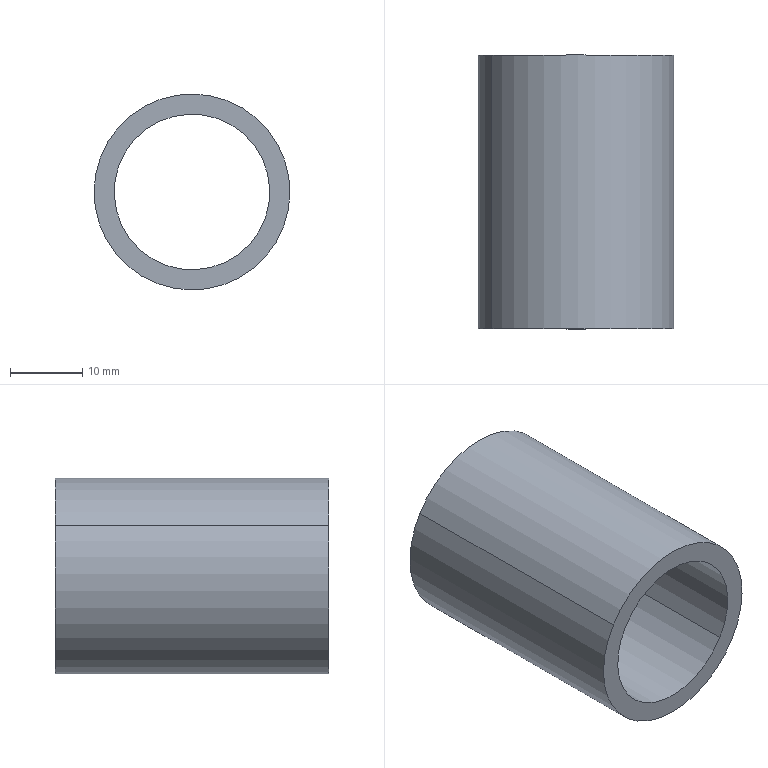Part | STEP file | [02]-12 | 1 solid | 6 faces | box 27.2 x 38 x 27.2 mm | volume 8156 mm3 | cylinder 4 | plane 2 | commonest cylinder face diameters 21.6 x2 27.2 x2
STEP:
#1=CARTESIAN_POINT('',(0.,0.,0.));
#2=DIRECTION('',(0.,0.,1.));
#3=DIRECTION('',(1.,0.,0.));
#4=AXIS2_PLACEMENT_3D('',#1,#2,#3);
#5=CARTESIAN_POINT('',(9.263,20.,-5.553));
#6=VERTEX_POINT('',#5);
#7=CARTESIAN_POINT('',(9.263,-18.,-5.553));
#8=VERTEX_POINT('',#7);
#9=CARTESIAN_POINT('',(9.263,20.,-5.553));
#10=DIRECTION('',(0.,-1.,0.));
#11=VECTOR('',#10,1.);
#12=LINE('',#9,#11);
#13=CARTESIAN_POINT('',(0.,20.,0.));
#14=DIRECTION('',(0.,-1.,0.));
#15=DIRECTION('',(0.8577,0.,-0.5142));
#16=AXIS2_PLACEMENT_3D('',#13,#14,#15);
#17=CYLINDRICAL_SURFACE('',#16,10.8);
#18=CARTESIAN_POINT('',(6.283,0.));
#19=DIRECTION('',(0.,1.));
#20=VECTOR('',#19,1.);
#21=LINE('',#18,#20);
#22=(GEOMETRIC_REPRESENTATION_CONTEXT(2)PARAMETRIC_REPRESENTATION_CONTEXT()REPRESENTATION_CONTEXT('',''));
#23=DEFINITIONAL_REPRESENTATION('',(#21),#22);
#24=PCURVE('',#17,#23);
#25=CARTESIAN_POINT('',(0.,20.,0.));
#26=DIRECTION('',(0.,-1.,0.));
#27=DIRECTION('',(0.8577,0.,-0.5142));
#28=AXIS2_PLACEMENT_3D('',#25,#26,#27);
#29=CYLINDRICAL_SURFACE('',#28,10.8);
#30=CARTESIAN_POINT('',(0.,0.));
#31=DIRECTION('',(0.,1.));
#32=VECTOR('',#31,1.);
#33=LINE('',#30,#32);
#34=(GEOMETRIC_REPRESENTATION_CONTEXT(2)PARAMETRIC_REPRESENTATION_CONTEXT()REPRESENTATION_CONTEXT('',''));
#35=DEFINITIONAL_REPRESENTATION('',(#33),#34);
#36=PCURVE('',#29,#35);
#37=SURFACE_CURVE('',#12,(#24,#36),.PCURVE_S1.);
#38=EDGE_CURVE('',#6,#8,#37,.T.);
#39=ORIENTED_EDGE('',*,*,#38,.T.);
#40=CARTESIAN_POINT('',(-9.263,-18.,5.553));
#41=VERTEX_POINT('',#40);
#42=CARTESIAN_POINT('',(0.,-18.,0.));
#43=DIRECTION('',(0.,1.,0.));
#44=DIRECTION('',(-0.8577,0.,0.5142));
#45=AXIS2_PLACEMENT_3D('',#42,#43,#44);
#46=CIRCLE('',#45,10.8);
#47=CARTESIAN_POINT('',(9.425,38.));
#48=DIRECTION('',(-1.,0.));
#49=VECTOR('',#48,1.);
#50=LINE('',#47,#49);
#51=(GEOMETRIC_REPRESENTATION_CONTEXT(2)PARAMETRIC_REPRESENTATION_CONTEXT()REPRESENTATION_CONTEXT('',''));
#52=DEFINITIONAL_REPRESENTATION('',(#50),#51);
#53=PCURVE('',#17,#52);
#54=CARTESIAN_POINT('',(0.,-18.,0.));
#55=DIRECTION('',(0.,-1.,0.));
#56=DIRECTION('',(0.8577,0.,-0.5142));
#57=AXIS2_PLACEMENT_3D('',#54,#55,#56);
#58=PLANE('',#57);
#59=CARTESIAN_POINT('',(-10.8,0.));
#60=CARTESIAN_POINT('',(-10.8,18.706));
#61=CARTESIAN_POINT('',(5.4,9.353));
#62=CARTESIAN_POINT('',(21.6,0.));
#63=CARTESIAN_POINT('',(5.4,-9.353));
#64=CARTESIAN_POINT('',(-10.8,-18.706));
#65=CARTESIAN_POINT('',(-10.8,0.));
#66=(BOUNDED_CURVE()B_SPLINE_CURVE(2,(#59,#60,#61,#62,#63,#64,#65),.UNSPECIFIED.,.T.,.F.)B_SPLINE_CURVE_WITH_KNOTS((1,2,2,2,2,1),(-2.094,0.,2.094,4.189,6.283,8.378),.UNSPECIFIED.)CURVE()GEOMETRIC_REPRESENTATION_ITEM()RATIONAL_B_SPLINE_CURVE((1.,0.5,1.,0.5,1.,0.5,1.))REPRESENTATION_ITEM(''));
#67=(GEOMETRIC_REPRESENTATION_CONTEXT(2)PARAMETRIC_REPRESENTATION_CONTEXT()REPRESENTATION_CONTEXT('',''));
#68=DEFINITIONAL_REPRESENTATION('',(#66),#67);
#69=PCURVE('',#58,#68);
#70=SURFACE_CURVE('',#46,(#53,#69),.PCURVE_S1.);
#71=EDGE_CURVE('',#8,#41,#70,.T.);
#72=ORIENTED_EDGE('',*,*,#71,.T.);
#73=CARTESIAN_POINT('',(-9.263,20.,5.553));
#74=VERTEX_POINT('',#73);
#75=CARTESIAN_POINT('',(-9.263,20.,5.553));
#76=DIRECTION('',(0.,-1.,0.));
#77=VECTOR('',#76,1.);
#78=LINE('',#75,#77);
#79=CARTESIAN_POINT('',(3.142,0.));
#80=DIRECTION('',(0.,1.));
#81=VECTOR('',#80,1.);
#82=LINE('',#79,#81);
#83=(GEOMETRIC_REPRESENTATION_CONTEXT(2)PARAMETRIC_REPRESENTATION_CONTEXT()REPRESENTATION_CONTEXT('',''));
#84=DEFINITIONAL_REPRESENTATION('',(#82),#83);
#85=PCURVE('',#17,#84);
#86=CARTESIAN_POINT('',(3.142,0.));
#87=DIRECTION('',(0.,1.));
#88=VECTOR('',#87,1.);
#89=LINE('',#86,#88);
#90=(GEOMETRIC_REPRESENTATION_CONTEXT(2)PARAMETRIC_REPRESENTATION_CONTEXT()REPRESENTATION_CONTEXT('',''));
#91=DEFINITIONAL_REPRESENTATION('',(#89),#90);
#92=PCURVE('',#29,#91);
#93=SURFACE_CURVE('',#78,(#85,#92),.PCURVE_S1.);
#94=EDGE_CURVE('',#74,#41,#93,.T.);
#95=ORIENTED_EDGE('',*,*,#94,.F.);
#96=CARTESIAN_POINT('',(0.,20.,0.));
#97=DIRECTION('',(0.,-1.,0.));
#98=DIRECTION('',(0.8577,0.,-0.5142));
#99=AXIS2_PLACEMENT_3D('',#96,#97,#98);
#100=CIRCLE('',#99,10.8);
#101=CARTESIAN_POINT('',(0.,0.));
#102=DIRECTION('',(1.,0.));
#103=VECTOR('',#102,1.);
#104=LINE('',#101,#103);
#105=(GEOMETRIC_REPRESENTATION_CONTEXT(2)PARAMETRIC_REPRESENTATION_CONTEXT()REPRESENTATION_CONTEXT('',''));
#106=DEFINITIONAL_REPRESENTATION('',(#104),#105);
#107=PCURVE('',#17,#106);
#108=CARTESIAN_POINT('',(0.,20.,0.));
#109=DIRECTION('',(0.,1.,0.));
#110=DIRECTION('',(-0.8577,0.,0.5142));
#111=AXIS2_PLACEMENT_3D('',#108,#109,#110);
#112=PLANE('',#111);
#113=CARTESIAN_POINT('',(-10.8,0.));
#114=CARTESIAN_POINT('',(-10.8,18.706));
#115=CARTESIAN_POINT('',(5.4,9.353));
#116=CARTESIAN_POINT('',(21.6,0.));
#117=CARTESIAN_POINT('',(5.4,-9.353));
#118=CARTESIAN_POINT('',(-10.8,-18.706));
#119=CARTESIAN_POINT('',(-10.8,0.));
#120=(BOUNDED_CURVE()B_SPLINE_CURVE(2,(#113,#114,#115,#116,#117,#118,#119),.UNSPECIFIED.,.T.,.F.)B_SPLINE_CURVE_WITH_KNOTS((1,2,2,2,2,1),(-2.094,0.,2.094,4.189,6.283,8.378),.UNSPECIFIED.)CURVE()GEOMETRIC_REPRESENTATION_ITEM()RATIONAL_B_SPLINE_CURVE((1.,0.5,1.,0.5,1.,0.5,1.))REPRESENTATION_ITEM(''));
#121=(GEOMETRIC_REPRESENTATION_CONTEXT(2)PARAMETRIC_REPRESENTATION_CONTEXT()REPRESENTATION_CONTEXT('',''));
#122=DEFINITIONAL_REPRESENTATION('',(#120),#121);
#123=PCURVE('',#112,#122);
#124=SURFACE_CURVE('',#100,(#107,#123),.PCURVE_S1.);
#125=EDGE_CURVE('',#74,#6,#124,.T.);
#126=ORIENTED_EDGE('',*,*,#125,.T.);
#127=EDGE_LOOP('',(#39,#72,#95,#126));
#128=FACE_BOUND('',#127,.F.);
#129=ADVANCED_FACE('',(#128),#17,.F.);
#130=CARTESIAN_POINT('',(11.665,20.,-6.993));
#131=VERTEX_POINT('',#130);
#132=CARTESIAN_POINT('',(-11.665,20.,6.993));
#133=VERTEX_POINT('',#132);
#134=CARTESIAN_POINT('',(0.,20.,0.));
#135=DIRECTION('',(0.,-1.,0.));
#136=DIRECTION('',(0.8577,0.,-0.5142));
#137=AXIS2_PLACEMENT_3D('',#134,#135,#136);
#138=CIRCLE('',#137,13.6);
#139=CARTESIAN_POINT('',(0.,20.,0.));
#140=DIRECTION('',(0.,-1.,0.));
#141=DIRECTION('',(0.8577,0.,-0.5142));
#142=AXIS2_PLACEMENT_3D('',#139,#140,#141);
#143=CYLINDRICAL_SURFACE('',#142,13.6);
#144=CARTESIAN_POINT('',(0.,0.));
#145=DIRECTION('',(1.,0.));
#146=VECTOR('',#145,1.);
#147=LINE('',#144,#146);
#148=(GEOMETRIC_REPRESENTATION_CONTEXT(2)PARAMETRIC_REPRESENTATION_CONTEXT()REPRESENTATION_CONTEXT('',''));
#149=DEFINITIONAL_REPRESENTATION('',(#147),#148);
#150=PCURVE('',#143,#149);
#151=CARTESIAN_POINT('',(-13.6,0.));
#152=CARTESIAN_POINT('',(-13.6,23.556));
#153=CARTESIAN_POINT('',(6.8,11.778));
#154=CARTESIAN_POINT('',(27.2,0.));
#155=CARTESIAN_POINT('',(6.8,-11.778));
#156=CARTESIAN_POINT('',(-13.6,-23.556));
#157=CARTESIAN_POINT('',(-13.6,0.));
#158=(BOUNDED_CURVE()B_SPLINE_CURVE(2,(#151,#152,#153,#154,#155,#156,#157),.UNSPECIFIED.,.T.,.F.)B_SPLINE_CURVE_WITH_KNOTS((1,2,2,2,2,1),(-2.094,0.,2.094,4.189,6.283,8.378),.UNSPECIFIED.)CURVE()GEOMETRIC_REPRESENTATION_ITEM()RATIONAL_B_SPLINE_CURVE((1.,0.5,1.,0.5,1.,0.5,1.))REPRESENTATION_ITEM(''));
#159=(GEOMETRIC_REPRESENTATION_CONTEXT(2)PARAMETRIC_REPRESENTATION_CONTEXT()REPRESENTATION_CONTEXT('',''));
#160=DEFINITIONAL_REPRESENTATION('',(#158),#159);
#161=PCURVE('',#112,#160);
#162=SURFACE_CURVE('',#138,(#150,#161),.PCURVE_S1.);
#163=EDGE_CURVE('',#131,#133,#162,.T.);
#164=ORIENTED_EDGE('',*,*,#163,.T.);
#165=CARTESIAN_POINT('',(-11.665,-18.,6.993));
#166=VERTEX_POINT('',#165);
#167=CARTESIAN_POINT('',(-11.665,20.,6.993));
#168=DIRECTION('',(0.,-1.,0.));
#169=VECTOR('',#168,1.);
#170=LINE('',#167,#169);
#171=CARTESIAN_POINT('',(3.142,0.));
#172=DIRECTION('',(0.,1.));
#173=VECTOR('',#172,1.);
#174=LINE('',#171,#173);
#175=(GEOMETRIC_REPRESENTATION_CONTEXT(2)PARAMETRIC_REPRESENTATION_CONTEXT()REPRESENTATION_CONTEXT('',''));
#176=DEFINITIONAL_REPRESENTATION('',(#174),#175);
#177=PCURVE('',#143,#176);
#178=CARTESIAN_POINT('',(0.,20.,0.));
#179=DIRECTION('',(0.,-1.,0.));
#180=DIRECTION('',(0.8577,0.,-0.5142));
#181=AXIS2_PLACEMENT_3D('',#178,#179,#180);
#182=CYLINDRICAL_SURFACE('',#181,13.6);
#183=CARTESIAN_POINT('',(3.142,0.));
#184=DIRECTION('',(0.,1.));
#185=VECTOR('',#184,1.);
#186=LINE('',#183,#185);
#187=(GEOMETRIC_REPRESENTATION_CONTEXT(2)PARAMETRIC_REPRESENTATION_CONTEXT()REPRESENTATION_CONTEXT('',''));
#188=DEFINITIONAL_REPRESENTATION('',(#186),#187);
#189=PCURVE('',#182,#188);
#190=SURFACE_CURVE('',#170,(#177,#189),.PCURVE_S1.);
#191=EDGE_CURVE('',#133,#166,#190,.T.);
#192=ORIENTED_EDGE('',*,*,#191,.T.);
#193=CARTESIAN_POINT('',(11.665,-18.,-6.993));
#194=VERTEX_POINT('',#193);
#195=CARTESIAN_POINT('',(0.,-18.,0.));
#196=DIRECTION('',(0.,1.,0.));
#197=DIRECTION('',(-0.8577,0.,0.5142));
#198=AXIS2_PLACEMENT_3D('',#195,#196,#197);
#199=CIRCLE('',#198,13.6);
#200=CARTESIAN_POINT('',(3.142,38.));
#201=DIRECTION('',(-1.,0.));
#202=VECTOR('',#201,1.);
#203=LINE('',#200,#202);
#204=(GEOMETRIC_REPRESENTATION_CONTEXT(2)PARAMETRIC_REPRESENTATION_CONTEXT()REPRESENTATION_CONTEXT('',''));
#205=DEFINITIONAL_REPRESENTATION('',(#203),#204);
#206=PCURVE('',#143,#205);
#207=CARTESIAN_POINT('',(-13.6,0.));
#208=CARTESIAN_POINT('',(-13.6,23.556));
#209=CARTESIAN_POINT('',(6.8,11.778));
#210=CARTESIAN_POINT('',(27.2,0.));
#211=CARTESIAN_POINT('',(6.8,-11.778));
#212=CARTESIAN_POINT('',(-13.6,-23.556));
#213=CARTESIAN_POINT('',(-13.6,0.));
#214=(BOUNDED_CURVE()B_SPLINE_CURVE(2,(#207,#208,#209,#210,#211,#212,#213),.UNSPECIFIED.,.T.,.F.)B_SPLINE_CURVE_WITH_KNOTS((1,2,2,2,2,1),(-2.094,0.,2.094,4.189,6.283,8.378),.UNSPECIFIED.)CURVE()GEOMETRIC_REPRESENTATION_ITEM()RATIONAL_B_SPLINE_CURVE((1.,0.5,1.,0.5,1.,0.5,1.))REPRESENTATION_ITEM(''));
#215=(GEOMETRIC_REPRESENTATION_CONTEXT(2)PARAMETRIC_REPRESENTATION_CONTEXT()REPRESENTATION_CONTEXT('',''));
#216=DEFINITIONAL_REPRESENTATION('',(#214),#215);
#217=PCURVE('',#58,#216);
#218=SURFACE_CURVE('',#199,(#206,#217),.PCURVE_S1.);
#219=EDGE_CURVE('',#166,#194,#218,.T.);
#220=ORIENTED_EDGE('',*,*,#219,.T.);
#221=CARTESIAN_POINT('',(11.665,20.,-6.993));
#222=DIRECTION('',(0.,-1.,0.));
#223=VECTOR('',#222,1.);
#224=LINE('',#221,#223);
#225=CARTESIAN_POINT('',(0.,0.));
#226=DIRECTION('',(0.,1.));
#227=VECTOR('',#226,1.);
#228=LINE('',#225,#227);
#229=(GEOMETRIC_REPRESENTATION_CONTEXT(2)PARAMETRIC_REPRESENTATION_CONTEXT()REPRESENTATION_CONTEXT('',''));
#230=DEFINITIONAL_REPRESENTATION('',(#228),#229);
#231=PCURVE('',#143,#230);
#232=CARTESIAN_POINT('',(6.283,0.));
#233=DIRECTION('',(0.,1.));
#234=VECTOR('',#233,1.);
#235=LINE('',#232,#234);
#236=(GEOMETRIC_REPRESENTATION_CONTEXT(2)PARAMETRIC_REPRESENTATION_CONTEXT()REPRESENTATION_CONTEXT('',''));
#237=DEFINITIONAL_REPRESENTATION('',(#235),#236);
#238=PCURVE('',#182,#237);
#239=SURFACE_CURVE('',#224,(#231,#238),.PCURVE_S1.);
#240=EDGE_CURVE('',#131,#194,#239,.T.);
#241=ORIENTED_EDGE('',*,*,#240,.F.);
#242=EDGE_LOOP('',(#164,#192,#220,#241));
#243=FACE_BOUND('',#242,.T.);
#244=ADVANCED_FACE('',(#243),#143,.T.);
#245=ORIENTED_EDGE('',*,*,#71,.T.);
#246=CARTESIAN_POINT('',(0.,-18.,0.));
#247=DIRECTION('',(0.,1.,0.));
#248=DIRECTION('',(-0.8577,0.,0.5142));
#249=AXIS2_PLACEMENT_3D('',#246,#247,#248);
#250=CIRCLE('',#249,10.8);
#251=CARTESIAN_POINT('',(-10.8,0.));
#252=CARTESIAN_POINT('',(-10.8,18.706));
#253=CARTESIAN_POINT('',(5.4,9.353));
#254=CARTESIAN_POINT('',(21.6,0.));
#255=CARTESIAN_POINT('',(5.4,-9.353));
#256=CARTESIAN_POINT('',(-10.8,-18.706));
#257=CARTESIAN_POINT('',(-10.8,0.));
#258=(BOUNDED_CURVE()B_SPLINE_CURVE(2,(#251,#252,#253,#254,#255,#256,#257),.UNSPECIFIED.,.T.,.F.)B_SPLINE_CURVE_WITH_KNOTS((1,2,2,2,2,1),(-2.094,0.,2.094,4.189,6.283,8.378),.UNSPECIFIED.)CURVE()GEOMETRIC_REPRESENTATION_ITEM()RATIONAL_B_SPLINE_CURVE((1.,0.5,1.,0.5,1.,0.5,1.))REPRESENTATION_ITEM(''));
#259=(GEOMETRIC_REPRESENTATION_CONTEXT(2)PARAMETRIC_REPRESENTATION_CONTEXT()REPRESENTATION_CONTEXT('',''));
#260=DEFINITIONAL_REPRESENTATION('',(#258),#259);
#261=PCURVE('',#58,#260);
#262=CARTESIAN_POINT('',(3.142,38.));
#263=DIRECTION('',(-1.,0.));
#264=VECTOR('',#263,1.);
#265=LINE('',#262,#264);
#266=(GEOMETRIC_REPRESENTATION_CONTEXT(2)PARAMETRIC_REPRESENTATION_CONTEXT()REPRESENTATION_CONTEXT('',''));
#267=DEFINITIONAL_REPRESENTATION('',(#265),#266);
#268=PCURVE('',#29,#267);
#269=SURFACE_CURVE('',#250,(#261,#268),.PCURVE_S1.);
#270=EDGE_CURVE('',#41,#8,#269,.T.);
#271=ORIENTED_EDGE('',*,*,#270,.T.);
#272=EDGE_LOOP('',(#245,#271));
#273=FACE_BOUND('',#272,.T.);
#274=CARTESIAN_POINT('',(0.,-18.,0.));
#275=DIRECTION('',(0.,1.,0.));
#276=DIRECTION('',(-0.8577,0.,0.5142));
#277=AXIS2_PLACEMENT_3D('',#274,#275,#276);
#278=CIRCLE('',#277,13.6);
#279=CARTESIAN_POINT('',(-13.6,0.));
#280=CARTESIAN_POINT('',(-13.6,23.556));
#281=CARTESIAN_POINT('',(6.8,11.778));
#282=CARTESIAN_POINT('',(27.2,0.));
#283=CARTESIAN_POINT('',(6.8,-11.778));
#284=CARTESIAN_POINT('',(-13.6,-23.556));
#285=CARTESIAN_POINT('',(-13.6,0.));
#286=(BOUNDED_CURVE()B_SPLINE_CURVE(2,(#279,#280,#281,#282,#283,#284,#285),.UNSPECIFIED.,.T.,.F.)B_SPLINE_CURVE_WITH_KNOTS((1,2,2,2,2,1),(-2.094,0.,2.094,4.189,6.283,8.378),.UNSPECIFIED.)CURVE()GEOMETRIC_REPRESENTATION_ITEM()RATIONAL_B_SPLINE_CURVE((1.,0.5,1.,0.5,1.,0.5,1.))REPRESENTATION_ITEM(''));
#287=(GEOMETRIC_REPRESENTATION_CONTEXT(2)PARAMETRIC_REPRESENTATION_CONTEXT()REPRESENTATION_CONTEXT('',''));
#288=DEFINITIONAL_REPRESENTATION('',(#286),#287);
#289=PCURVE('',#58,#288);
#290=CARTESIAN_POINT('',(9.425,38.));
#291=DIRECTION('',(-1.,0.));
#292=VECTOR('',#291,1.);
#293=LINE('',#290,#292);
#294=(GEOMETRIC_REPRESENTATION_CONTEXT(2)PARAMETRIC_REPRESENTATION_CONTEXT()REPRESENTATION_CONTEXT('',''));
#295=DEFINITIONAL_REPRESENTATION('',(#293),#294);
#296=PCURVE('',#182,#295);
#297=SURFACE_CURVE('',#278,(#289,#296),.PCURVE_S1.);
#298=EDGE_CURVE('',#194,#166,#297,.T.);
#299=ORIENTED_EDGE('',*,*,#298,.F.);
#300=ORIENTED_EDGE('',*,*,#219,.F.);
#301=EDGE_LOOP('',(#299,#300));
#302=FACE_BOUND('',#301,.T.);
#303=ADVANCED_FACE('',(#273,#302),#58,.T.);
#304=CARTESIAN_POINT('',(0.,20.,0.));
#305=DIRECTION('',(0.,-1.,0.));
#306=DIRECTION('',(0.8577,0.,-0.5142));
#307=AXIS2_PLACEMENT_3D('',#304,#305,#306);
#308=CIRCLE('',#307,10.8);
#309=CARTESIAN_POINT('',(-10.8,0.));
#310=CARTESIAN_POINT('',(-10.8,18.706));
#311=CARTESIAN_POINT('',(5.4,9.353));
#312=CARTESIAN_POINT('',(21.6,0.));
#313=CARTESIAN_POINT('',(5.4,-9.353));
#314=CARTESIAN_POINT('',(-10.8,-18.706));
#315=CARTESIAN_POINT('',(-10.8,0.));
#316=(BOUNDED_CURVE()B_SPLINE_CURVE(2,(#309,#310,#311,#312,#313,#314,#315),.UNSPECIFIED.,.T.,.F.)B_SPLINE_CURVE_WITH_KNOTS((1,2,2,2,2,1),(-2.094,0.,2.094,4.189,6.283,8.378),.UNSPECIFIED.)CURVE()GEOMETRIC_REPRESENTATION_ITEM()RATIONAL_B_SPLINE_CURVE((1.,0.5,1.,0.5,1.,0.5,1.))REPRESENTATION_ITEM(''));
#317=(GEOMETRIC_REPRESENTATION_CONTEXT(2)PARAMETRIC_REPRESENTATION_CONTEXT()REPRESENTATION_CONTEXT('',''));
#318=DEFINITIONAL_REPRESENTATION('',(#316),#317);
#319=PCURVE('',#112,#318);
#320=CARTESIAN_POINT('',(0.,0.));
#321=DIRECTION('',(1.,0.));
#322=VECTOR('',#321,1.);
#323=LINE('',#320,#322);
#324=(GEOMETRIC_REPRESENTATION_CONTEXT(2)PARAMETRIC_REPRESENTATION_CONTEXT()REPRESENTATION_CONTEXT('',''));
#325=DEFINITIONAL_REPRESENTATION('',(#323),#324);
#326=PCURVE('',#29,#325);
#327=SURFACE_CURVE('',#308,(#319,#326),.PCURVE_S1.);
#328=EDGE_CURVE('',#6,#74,#327,.T.);
#329=ORIENTED_EDGE('',*,*,#328,.T.);
#330=ORIENTED_EDGE('',*,*,#125,.T.);
#331=EDGE_LOOP('',(#329,#330));
#332=FACE_BOUND('',#331,.T.);
#333=ORIENTED_EDGE('',*,*,#163,.F.);
#334=CARTESIAN_POINT('',(0.,20.,0.));
#335=DIRECTION('',(0.,-1.,0.));
#336=DIRECTION('',(0.8577,0.,-0.5142));
#337=AXIS2_PLACEMENT_3D('',#334,#335,#336);
#338=CIRCLE('',#337,13.6);
#339=CARTESIAN_POINT('',(-13.6,0.));
#340=CARTESIAN_POINT('',(-13.6,23.556));
#341=CARTESIAN_POINT('',(6.8,11.778));
#342=CARTESIAN_POINT('',(27.2,0.));
#343=CARTESIAN_POINT('',(6.8,-11.778));
#344=CARTESIAN_POINT('',(-13.6,-23.556));
#345=CARTESIAN_POINT('',(-13.6,0.));
#346=(BOUNDED_CURVE()B_SPLINE_CURVE(2,(#339,#340,#341,#342,#343,#344,#345),.UNSPECIFIED.,.T.,.F.)B_SPLINE_CURVE_WITH_KNOTS((1,2,2,2,2,1),(-2.094,0.,2.094,4.189,6.283,8.378),.UNSPECIFIED.)CURVE()GEOMETRIC_REPRESENTATION_ITEM()RATIONAL_B_SPLINE_CURVE((1.,0.5,1.,0.5,1.,0.5,1.))REPRESENTATION_ITEM(''));
#347=(GEOMETRIC_REPRESENTATION_CONTEXT(2)PARAMETRIC_REPRESENTATION_CONTEXT()REPRESENTATION_CONTEXT('',''));
#348=DEFINITIONAL_REPRESENTATION('',(#346),#347);
#349=PCURVE('',#112,#348);
#350=CARTESIAN_POINT('',(0.,0.));
#351=DIRECTION('',(1.,0.));
#352=VECTOR('',#351,1.);
#353=LINE('',#350,#352);
#354=(GEOMETRIC_REPRESENTATION_CONTEXT(2)PARAMETRIC_REPRESENTATION_CONTEXT()REPRESENTATION_CONTEXT('',''));
#355=DEFINITIONAL_REPRESENTATION('',(#353),#354);
#356=PCURVE('',#182,#355);
#357=SURFACE_CURVE('',#338,(#349,#356),.PCURVE_S1.);
#358=EDGE_CURVE('',#133,#131,#357,.T.);
#359=ORIENTED_EDGE('',*,*,#358,.F.);
#360=EDGE_LOOP('',(#333,#359));
#361=FACE_BOUND('',#360,.T.);
#362=ADVANCED_FACE('',(#332,#361),#112,.T.);
#363=ORIENTED_EDGE('',*,*,#191,.F.);
#364=ORIENTED_EDGE('',*,*,#358,.T.);
#365=ORIENTED_EDGE('',*,*,#240,.T.);
#366=ORIENTED_EDGE('',*,*,#298,.T.);
#367=EDGE_LOOP('',(#363,#364,#365,#366));
#368=FACE_BOUND('',#367,.T.);
#369=ADVANCED_FACE('',(#368),#182,.T.);
#370=ORIENTED_EDGE('',*,*,#270,.T.);
#371=ORIENTED_EDGE('',*,*,#38,.F.);
#372=ORIENTED_EDGE('',*,*,#328,.T.);
#373=ORIENTED_EDGE('',*,*,#94,.T.);
#374=EDGE_LOOP('',(#370,#371,#372,#373));
#375=FACE_BOUND('',#374,.F.);
#376=ADVANCED_FACE('',(#375),#29,.F.);
#377=CLOSED_SHELL('',(#129,#244,#303,#362,#369,#376));
#378=MANIFOLD_SOLID_BREP('',#377);
#379=(LENGTH_UNIT()NAMED_UNIT(*)SI_UNIT(.MILLI.,.METRE.));
#380=UNCERTAINTY_MEASURE_WITH_UNIT(LENGTH_MEASURE(0.0000001),#379,'','');
#381=(NAMED_UNIT(*)PLANE_ANGLE_UNIT()SI_UNIT($,.RADIAN.));
#382=(NAMED_UNIT(*)SI_UNIT($,.STERADIAN.)SOLID_ANGLE_UNIT());
#383=(GEOMETRIC_REPRESENTATION_CONTEXT(3)GLOBAL_UNCERTAINTY_ASSIGNED_CONTEXT((#380))GLOBAL_UNIT_ASSIGNED_CONTEXT((#379,#381,#382))REPRESENTATION_CONTEXT('',''));
#384=ADVANCED_BREP_SHAPE_REPRESENTATION('',(#4,#378),#383);